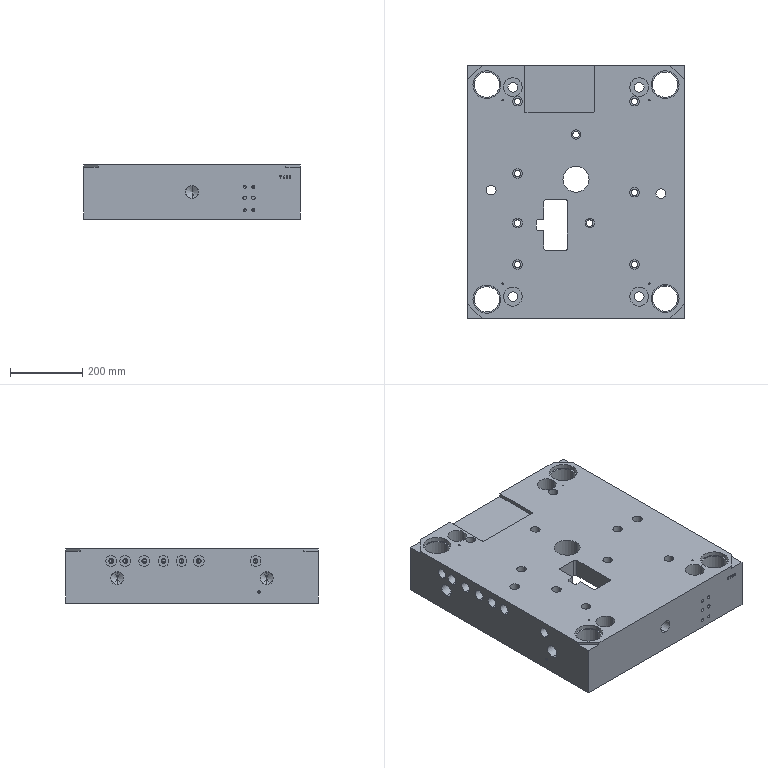Part | Creo | 5 solids | 953 faces | box 600 x 700 x 150 mm | volume 37038088 mm3 | cylinder 469 | plane 221 | cone 201 | other 42 | torus 16 | spline 4 | commonest cylinder face diameters 10 x76 8.5 x38 13 x32 19.5 x32 30 x32 5 x24